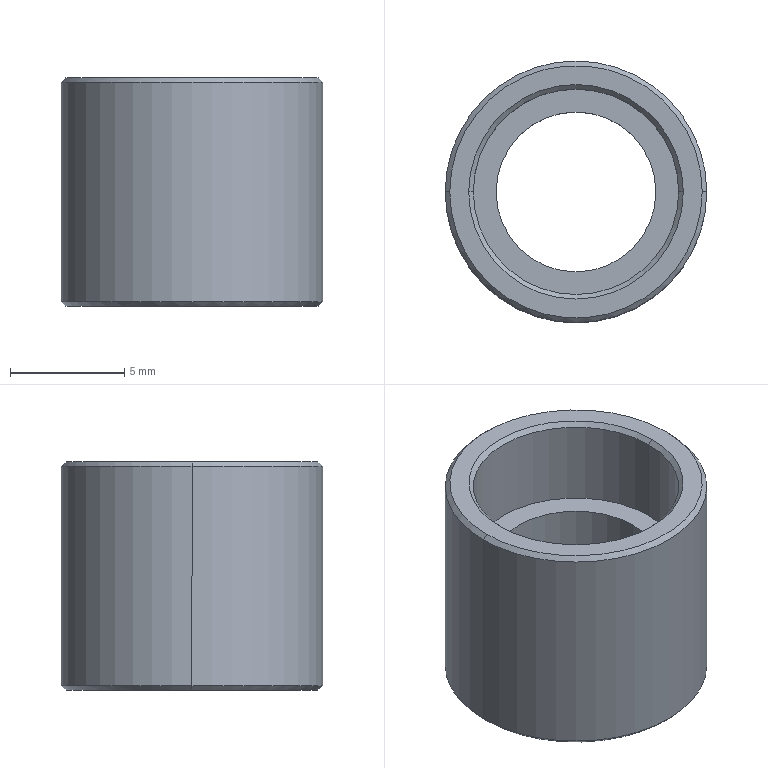Part | SolidWorks | features Revolution 1 | 1 solid | 20 faces | box 11.46 x 11.46 x 10 mm | volume 442.998 mm3 | cylinder 8 | cone 8 | plane 4 | commonest cylinder face diameters 9 x4 7 x2 11.46 x2
STEP:
#1=CARTESIAN_POINT('',(-4.5,0.,-9.8));
#2=VERTEX_POINT('',#1);
#3=CARTESIAN_POINT('',(4.5,0.,-9.8));
#4=VERTEX_POINT('',#3);
#5=CARTESIAN_POINT('',(0.,0.,-9.8));
#6=DIRECTION('',(0.,0.,1.));
#7=DIRECTION('',(1.,0.,0.));
#8=AXIS2_PLACEMENT_3D('',#5,#6,#7);
#9=CIRCLE('',#8,4.5);
#10=EDGE_CURVE('',#2,#4,#9,.T.);
#11=ORIENTED_EDGE('',*,*,#10,.F.);
#12=CARTESIAN_POINT('',(-4.5,0.,-6.));
#13=VERTEX_POINT('',#12);
#14=CARTESIAN_POINT('',(-4.5,0.,0.));
#15=DIRECTION('',(0.,0.,1.));
#16=VECTOR('',#15,1000.);
#17=LINE('',#14,#16);
#18=EDGE_CURVE('',#2,#13,#17,.T.);
#19=ORIENTED_EDGE('',*,*,#18,.T.);
#20=CARTESIAN_POINT('',(4.5,0.,-6.));
#21=VERTEX_POINT('',#20);
#22=CARTESIAN_POINT('',(0.,0.,-6.));
#23=DIRECTION('',(0.,0.,1.));
#24=DIRECTION('',(1.,0.,0.));
#25=AXIS2_PLACEMENT_3D('',#22,#23,#24);
#26=CIRCLE('',#25,4.5);
#27=EDGE_CURVE('',#13,#21,#26,.T.);
#28=ORIENTED_EDGE('',*,*,#27,.T.);
#29=CARTESIAN_POINT('',(4.5,0.,0.));
#30=DIRECTION('',(0.,0.,1.));
#31=VECTOR('',#30,1000.);
#32=LINE('',#29,#31);
#33=EDGE_CURVE('',#4,#21,#32,.T.);
#34=ORIENTED_EDGE('',*,*,#33,.F.);
#35=EDGE_LOOP('',(#11,#19,#28,#34));
#36=FACE_OUTER_BOUND('',#35,.T.);
#37=CARTESIAN_POINT('',(0.,0.,0.));
#38=DIRECTION('',(0.,0.,1.));
#39=DIRECTION('',(1.,0.,0.));
#40=AXIS2_PLACEMENT_3D('',#37,#38,#39);
#41=CYLINDRICAL_SURFACE('',#40,4.5);
#42=ADVANCED_FACE('',(#36),#41,.F.);
#43=ORIENTED_EDGE('',*,*,#10,.T.);
#44=CARTESIAN_POINT('',(4.7,0.,-10.));
#45=VERTEX_POINT('',#44);
#46=CARTESIAN_POINT('',(4.7,0.,-10.));
#47=DIRECTION('',(0.7071,0.,-0.7071));
#48=VECTOR('',#47,1000.);
#49=LINE('',#46,#48);
#50=EDGE_CURVE('',#4,#45,#49,.T.);
#51=ORIENTED_EDGE('',*,*,#50,.T.);
#52=CARTESIAN_POINT('',(-4.7,0.,-10.));
#53=VERTEX_POINT('',#52);
#54=CARTESIAN_POINT('',(0.,0.,-10.));
#55=DIRECTION('',(0.,0.,1.));
#56=DIRECTION('',(1.,0.,0.));
#57=AXIS2_PLACEMENT_3D('',#54,#55,#56);
#58=CIRCLE('',#57,4.7);
#59=EDGE_CURVE('',#53,#45,#58,.T.);
#60=ORIENTED_EDGE('',*,*,#59,.F.);
#61=CARTESIAN_POINT('',(-4.7,0.,-10.));
#62=DIRECTION('',(-0.7071,0.,-0.7071));
#63=VECTOR('',#62,1000.);
#64=LINE('',#61,#63);
#65=EDGE_CURVE('',#2,#53,#64,.T.);
#66=ORIENTED_EDGE('',*,*,#65,.F.);
#67=EDGE_LOOP('',(#43,#51,#60,#66));
#68=FACE_OUTER_BOUND('',#67,.T.);
#69=CARTESIAN_POINT('',(0.,0.,-10.));
#70=DIRECTION('',(0.,0.,-1.));
#71=DIRECTION('',(-1.,0.,0.));
#72=AXIS2_PLACEMENT_3D('',#69,#70,#71);
#73=CONICAL_SURFACE('',#72,4.7,0.7854);
#74=ADVANCED_FACE('',(#68),#73,.F.);
#75=CARTESIAN_POINT('',(5.53,0.,-10.));
#76=VERTEX_POINT('',#75);
#77=CARTESIAN_POINT('',(-5.53,0.,-10.));
#78=VERTEX_POINT('',#77);
#79=CARTESIAN_POINT('',(0.,0.,-10.));
#80=DIRECTION('',(0.,0.,1.));
#81=DIRECTION('',(1.,0.,0.));
#82=AXIS2_PLACEMENT_3D('',#79,#80,#81);
#83=CIRCLE('',#82,5.53);
#84=EDGE_CURVE('',#76,#78,#83,.T.);
#85=ORIENTED_EDGE('',*,*,#84,.T.);
#86=CARTESIAN_POINT('',(-5.73,0.,-9.8));
#87=VERTEX_POINT('',#86);
#88=CARTESIAN_POINT('',(-5.73,0.,-9.8));
#89=DIRECTION('',(-0.7071,0.,0.7071));
#90=VECTOR('',#89,1000.);
#91=LINE('',#88,#90);
#92=EDGE_CURVE('',#78,#87,#91,.T.);
#93=ORIENTED_EDGE('',*,*,#92,.T.);
#94=CARTESIAN_POINT('',(5.73,0.,-9.8));
#95=VERTEX_POINT('',#94);
#96=CARTESIAN_POINT('',(0.,0.,-9.8));
#97=DIRECTION('',(0.,0.,1.));
#98=DIRECTION('',(1.,0.,0.));
#99=AXIS2_PLACEMENT_3D('',#96,#97,#98);
#100=CIRCLE('',#99,5.73);
#101=EDGE_CURVE('',#95,#87,#100,.T.);
#102=ORIENTED_EDGE('',*,*,#101,.F.);
#103=CARTESIAN_POINT('',(5.73,0.,-9.8));
#104=DIRECTION('',(0.7071,0.,0.7071));
#105=VECTOR('',#104,1000.);
#106=LINE('',#103,#105);
#107=EDGE_CURVE('',#76,#95,#106,.T.);
#108=ORIENTED_EDGE('',*,*,#107,.F.);
#109=EDGE_LOOP('',(#85,#93,#102,#108));
#110=FACE_OUTER_BOUND('',#109,.T.);
#111=CARTESIAN_POINT('',(0.,0.,-9.8));
#112=DIRECTION('',(0.,0.,1.));
#113=DIRECTION('',(1.,0.,0.));
#114=AXIS2_PLACEMENT_3D('',#111,#112,#113);
#115=CONICAL_SURFACE('',#114,5.73,0.7854);
#116=ADVANCED_FACE('',(#110),#115,.T.);
#117=ORIENTED_EDGE('',*,*,#101,.T.);
#118=CARTESIAN_POINT('',(-5.73,0.,-0.2));
#119=VERTEX_POINT('',#118);
#120=CARTESIAN_POINT('',(-5.73,0.,0.));
#121=DIRECTION('',(0.,0.,1.));
#122=VECTOR('',#121,1000.);
#123=LINE('',#120,#122);
#124=EDGE_CURVE('',#87,#119,#123,.T.);
#125=ORIENTED_EDGE('',*,*,#124,.T.);
#126=CARTESIAN_POINT('',(5.73,0.,-0.2));
#127=VERTEX_POINT('',#126);
#128=CARTESIAN_POINT('',(0.,0.,-0.2));
#129=DIRECTION('',(0.,0.,1.));
#130=DIRECTION('',(1.,0.,0.));
#131=AXIS2_PLACEMENT_3D('',#128,#129,#130);
#132=CIRCLE('',#131,5.73);
#133=EDGE_CURVE('',#127,#119,#132,.T.);
#134=ORIENTED_EDGE('',*,*,#133,.F.);
#135=CARTESIAN_POINT('',(5.73,0.,0.));
#136=DIRECTION('',(0.,0.,1.));
#137=VECTOR('',#136,1000.);
#138=LINE('',#135,#137);
#139=EDGE_CURVE('',#95,#127,#138,.T.);
#140=ORIENTED_EDGE('',*,*,#139,.F.);
#141=EDGE_LOOP('',(#117,#125,#134,#140));
#142=FACE_OUTER_BOUND('',#141,.T.);
#143=CARTESIAN_POINT('',(0.,0.,0.));
#144=DIRECTION('',(0.,0.,1.));
#145=DIRECTION('',(1.,0.,0.));
#146=AXIS2_PLACEMENT_3D('',#143,#144,#145);
#147=CYLINDRICAL_SURFACE('',#146,5.73);
#148=ADVANCED_FACE('',(#142),#147,.T.);
#149=CARTESIAN_POINT('',(5.53,0.,0.));
#150=VERTEX_POINT('',#149);
#151=CARTESIAN_POINT('',(-5.53,0.,0.));
#152=VERTEX_POINT('',#151);
#153=CARTESIAN_POINT('',(0.,0.,0.));
#154=DIRECTION('',(0.,0.,1.));
#155=DIRECTION('',(1.,0.,0.));
#156=AXIS2_PLACEMENT_3D('',#153,#154,#155);
#157=CIRCLE('',#156,5.53);
#158=EDGE_CURVE('',#150,#152,#157,.T.);
#159=ORIENTED_EDGE('',*,*,#158,.F.);
#160=CARTESIAN_POINT('',(5.53,0.,0.));
#161=DIRECTION('',(0.7071,0.,-0.7071));
#162=VECTOR('',#161,1000.);
#163=LINE('',#160,#162);
#164=EDGE_CURVE('',#150,#127,#163,.T.);
#165=ORIENTED_EDGE('',*,*,#164,.T.);
#166=ORIENTED_EDGE('',*,*,#133,.T.);
#167=CARTESIAN_POINT('',(-5.53,0.,0.));
#168=DIRECTION('',(-0.7071,0.,-0.7071));
#169=VECTOR('',#168,1000.);
#170=LINE('',#167,#169);
#171=EDGE_CURVE('',#152,#119,#170,.T.);
#172=ORIENTED_EDGE('',*,*,#171,.F.);
#173=EDGE_LOOP('',(#159,#165,#166,#172));
#174=FACE_OUTER_BOUND('',#173,.T.);
#175=CARTESIAN_POINT('',(0.,0.,0.));
#176=DIRECTION('',(0.,0.,-1.));
#177=DIRECTION('',(-1.,0.,0.));
#178=AXIS2_PLACEMENT_3D('',#175,#176,#177);
#179=CONICAL_SURFACE('',#178,5.53,0.7854);
#180=ADVANCED_FACE('',(#174),#179,.T.);
#181=CARTESIAN_POINT('',(-4.5,0.,-0.2));
#182=VERTEX_POINT('',#181);
#183=CARTESIAN_POINT('',(4.5,0.,-0.2));
#184=VERTEX_POINT('',#183);
#185=CARTESIAN_POINT('',(0.,0.,-0.2));
#186=DIRECTION('',(0.,0.,1.));
#187=DIRECTION('',(1.,0.,0.));
#188=AXIS2_PLACEMENT_3D('',#185,#186,#187);
#189=CIRCLE('',#188,4.5);
#190=EDGE_CURVE('',#182,#184,#189,.T.);
#191=ORIENTED_EDGE('',*,*,#190,.F.);
#192=CARTESIAN_POINT('',(-4.7,0.,0.));
#193=VERTEX_POINT('',#192);
#194=CARTESIAN_POINT('',(-4.5,0.,-0.2));
#195=DIRECTION('',(-0.7071,0.,0.7071));
#196=VECTOR('',#195,1000.);
#197=LINE('',#194,#196);
#198=EDGE_CURVE('',#182,#193,#197,.T.);
#199=ORIENTED_EDGE('',*,*,#198,.T.);
#200=CARTESIAN_POINT('',(4.7,0.,0.));
#201=VERTEX_POINT('',#200);
#202=CARTESIAN_POINT('',(0.,0.,0.));
#203=DIRECTION('',(0.,0.,1.));
#204=DIRECTION('',(1.,0.,0.));
#205=AXIS2_PLACEMENT_3D('',#202,#203,#204);
#206=CIRCLE('',#205,4.7);
#207=EDGE_CURVE('',#193,#201,#206,.T.);
#208=ORIENTED_EDGE('',*,*,#207,.T.);
#209=CARTESIAN_POINT('',(4.5,0.,-0.2));
#210=DIRECTION('',(0.7071,0.,0.7071));
#211=VECTOR('',#210,1000.);
#212=LINE('',#209,#211);
#213=EDGE_CURVE('',#184,#201,#212,.T.);
#214=ORIENTED_EDGE('',*,*,#213,.F.);
#215=EDGE_LOOP('',(#191,#199,#208,#214));
#216=FACE_OUTER_BOUND('',#215,.T.);
#217=CARTESIAN_POINT('',(0.,0.,-0.2));
#218=DIRECTION('',(0.,0.,1.));
#219=DIRECTION('',(1.,0.,0.));
#220=AXIS2_PLACEMENT_3D('',#217,#218,#219);
#221=CONICAL_SURFACE('',#220,4.5,0.7854);
#222=ADVANCED_FACE('',(#216),#221,.F.);
#223=CARTESIAN_POINT('',(-4.5,0.,-4.));
#224=VERTEX_POINT('',#223);
#225=CARTESIAN_POINT('',(4.5,0.,-4.));
#226=VERTEX_POINT('',#225);
#227=CARTESIAN_POINT('',(0.,0.,-4.));
#228=DIRECTION('',(0.,0.,1.));
#229=DIRECTION('',(1.,0.,0.));
#230=AXIS2_PLACEMENT_3D('',#227,#228,#229);
#231=CIRCLE('',#230,4.5);
#232=EDGE_CURVE('',#224,#226,#231,.T.);
#233=ORIENTED_EDGE('',*,*,#232,.F.);
#234=CARTESIAN_POINT('',(-4.5,0.,0.));
#235=DIRECTION('',(0.,0.,1.));
#236=VECTOR('',#235,1000.);
#237=LINE('',#234,#236);
#238=EDGE_CURVE('',#224,#182,#237,.T.);
#239=ORIENTED_EDGE('',*,*,#238,.T.);
#240=ORIENTED_EDGE('',*,*,#190,.T.);
#241=CARTESIAN_POINT('',(4.5,0.,0.));
#242=DIRECTION('',(0.,0.,1.));
#243=VECTOR('',#242,1000.);
#244=LINE('',#241,#243);
#245=EDGE_CURVE('',#226,#184,#244,.T.);
#246=ORIENTED_EDGE('',*,*,#245,.F.);
#247=EDGE_LOOP('',(#233,#239,#240,#246));
#248=FACE_OUTER_BOUND('',#247,.T.);
#249=CARTESIAN_POINT('',(0.,0.,0.));
#250=DIRECTION('',(0.,0.,1.));
#251=DIRECTION('',(1.,0.,0.));
#252=AXIS2_PLACEMENT_3D('',#249,#250,#251);
#253=CYLINDRICAL_SURFACE('',#252,4.5);
#254=ADVANCED_FACE('',(#248),#253,.F.);
#255=CARTESIAN_POINT('',(-3.5,0.,-6.));
#256=VERTEX_POINT('',#255);
#257=CARTESIAN_POINT('',(3.5,0.,-6.));
#258=VERTEX_POINT('',#257);
#259=CARTESIAN_POINT('',(0.,0.,-6.));
#260=DIRECTION('',(0.,0.,1.));
#261=DIRECTION('',(1.,0.,0.));
#262=AXIS2_PLACEMENT_3D('',#259,#260,#261);
#263=CIRCLE('',#262,3.5);
#264=EDGE_CURVE('',#256,#258,#263,.T.);
#265=ORIENTED_EDGE('',*,*,#264,.F.);
#266=CARTESIAN_POINT('',(-3.5,0.,-4.));
#267=VERTEX_POINT('',#266);
#268=CARTESIAN_POINT('',(-3.5,0.,0.));
#269=DIRECTION('',(0.,0.,1.));
#270=VECTOR('',#269,1000.);
#271=LINE('',#268,#270);
#272=EDGE_CURVE('',#256,#267,#271,.T.);
#273=ORIENTED_EDGE('',*,*,#272,.T.);
#274=CARTESIAN_POINT('',(3.5,0.,-4.));
#275=VERTEX_POINT('',#274);
#276=CARTESIAN_POINT('',(0.,0.,-4.));
#277=DIRECTION('',(0.,0.,1.));
#278=DIRECTION('',(1.,0.,0.));
#279=AXIS2_PLACEMENT_3D('',#276,#277,#278);
#280=CIRCLE('',#279,3.5);
#281=EDGE_CURVE('',#267,#275,#280,.T.);
#282=ORIENTED_EDGE('',*,*,#281,.T.);
#283=CARTESIAN_POINT('',(3.5,0.,0.));
#284=DIRECTION('',(0.,0.,1.));
#285=VECTOR('',#284,1000.);
#286=LINE('',#283,#285);
#287=EDGE_CURVE('',#258,#275,#286,.T.);
#288=ORIENTED_EDGE('',*,*,#287,.F.);
#289=EDGE_LOOP('',(#265,#273,#282,#288));
#290=FACE_OUTER_BOUND('',#289,.T.);
#291=CARTESIAN_POINT('',(0.,0.,0.));
#292=DIRECTION('',(0.,0.,1.));
#293=DIRECTION('',(1.,0.,0.));
#294=AXIS2_PLACEMENT_3D('',#291,#292,#293);
#295=CYLINDRICAL_SURFACE('',#294,3.5);
#296=ADVANCED_FACE('',(#290),#295,.F.);
#297=CARTESIAN_POINT('',(0.,0.,-6.));
#298=DIRECTION('',(0.,0.,1.));
#299=DIRECTION('',(1.,0.,0.));
#300=AXIS2_PLACEMENT_3D('',#297,#298,#299);
#301=CIRCLE('',#300,3.5);
#302=EDGE_CURVE('',#258,#256,#301,.T.);
#303=ORIENTED_EDGE('',*,*,#302,.T.);
#304=ORIENTED_EDGE('',*,*,#264,.T.);
#305=EDGE_LOOP('',(#303,#304));
#306=FACE_BOUND('',#305,.T.);
#307=CARTESIAN_POINT('',(0.,0.,-6.));
#308=DIRECTION('',(0.,0.,1.));
#309=DIRECTION('',(1.,0.,0.));
#310=AXIS2_PLACEMENT_3D('',#307,#308,#309);
#311=CIRCLE('',#310,4.5);
#312=EDGE_CURVE('',#21,#13,#311,.T.);
#313=ORIENTED_EDGE('',*,*,#312,.F.);
#314=ORIENTED_EDGE('',*,*,#27,.F.);
#315=EDGE_LOOP('',(#313,#314));
#316=FACE_OUTER_BOUND('',#315,.T.);
#317=CARTESIAN_POINT('',(4.5,0.,-6.));
#318=DIRECTION('',(0.,0.,-1.));
#319=DIRECTION('',(-1.,0.,0.));
#320=AXIS2_PLACEMENT_3D('',#317,#318,#319);
#321=PLANE('',#320);
#322=ADVANCED_FACE('',(#306,#316),#321,.T.);
#323=ORIENTED_EDGE('',*,*,#272,.F.);
#324=ORIENTED_EDGE('',*,*,#302,.F.);
#325=ORIENTED_EDGE('',*,*,#287,.T.);
#326=CARTESIAN_POINT('',(0.,0.,-4.));
#327=DIRECTION('',(0.,0.,1.));
#328=DIRECTION('',(1.,0.,0.));
#329=AXIS2_PLACEMENT_3D('',#326,#327,#328);
#330=CIRCLE('',#329,3.5);
#331=EDGE_CURVE('',#275,#267,#330,.T.);
#332=ORIENTED_EDGE('',*,*,#331,.T.);
#333=EDGE_LOOP('',(#323,#324,#325,#332));
#334=FACE_OUTER_BOUND('',#333,.T.);
#335=CARTESIAN_POINT('',(0.,0.,0.));
#336=DIRECTION('',(0.,0.,1.));
#337=DIRECTION('',(1.,0.,0.));
#338=AXIS2_PLACEMENT_3D('',#335,#336,#337);
#339=CYLINDRICAL_SURFACE('',#338,3.5);
#340=ADVANCED_FACE('',(#334),#339,.F.);
#341=CARTESIAN_POINT('',(0.,0.,-4.));
#342=DIRECTION('',(0.,0.,1.));
#343=DIRECTION('',(1.,0.,0.));
#344=AXIS2_PLACEMENT_3D('',#341,#342,#343);
#345=CIRCLE('',#344,4.5);
#346=EDGE_CURVE('',#226,#224,#345,.T.);
#347=ORIENTED_EDGE('',*,*,#346,.T.);
#348=ORIENTED_EDGE('',*,*,#232,.T.);
#349=EDGE_LOOP('',(#347,#348));
#350=FACE_OUTER_BOUND('',#349,.T.);
#351=ORIENTED_EDGE('',*,*,#331,.F.);
#352=ORIENTED_EDGE('',*,*,#281,.F.);
#353=EDGE_LOOP('',(#351,#352));
#354=FACE_BOUND('',#353,.T.);
#355=CARTESIAN_POINT('',(3.5,0.,-4.));
#356=DIRECTION('',(0.,0.,1.));
#357=DIRECTION('',(1.,0.,0.));
#358=AXIS2_PLACEMENT_3D('',#355,#356,#357);
#359=PLANE('',#358);
#360=ADVANCED_FACE('',(#350,#354),#359,.T.);
#361=ORIENTED_EDGE('',*,*,#238,.F.);
#362=ORIENTED_EDGE('',*,*,#346,.F.);
#363=ORIENTED_EDGE('',*,*,#245,.T.);
#364=CARTESIAN_POINT('',(0.,0.,-0.2));
#365=DIRECTION('',(0.,0.,1.));
#366=DIRECTION('',(1.,0.,0.));
#367=AXIS2_PLACEMENT_3D('',#364,#365,#366);
#368=CIRCLE('',#367,4.5);
#369=EDGE_CURVE('',#184,#182,#368,.T.);
#370=ORIENTED_EDGE('',*,*,#369,.T.);
#371=EDGE_LOOP('',(#361,#362,#363,#370));
#372=FACE_OUTER_BOUND('',#371,.T.);
#373=CARTESIAN_POINT('',(0.,0.,0.));
#374=DIRECTION('',(0.,0.,1.));
#375=DIRECTION('',(1.,0.,0.));
#376=AXIS2_PLACEMENT_3D('',#373,#374,#375);
#377=CYLINDRICAL_SURFACE('',#376,4.5);
#378=ADVANCED_FACE('',(#372),#377,.F.);
#379=ORIENTED_EDGE('',*,*,#198,.F.);
#380=ORIENTED_EDGE('',*,*,#369,.F.);
#381=ORIENTED_EDGE('',*,*,#213,.T.);
#382=CARTESIAN_POINT('',(0.,0.,0.));
#383=DIRECTION('',(0.,0.,1.));
#384=DIRECTION('',(1.,0.,0.));
#385=AXIS2_PLACEMENT_3D('',#382,#383,#384);
#386=CIRCLE('',#385,4.7);
#387=EDGE_CURVE('',#201,#193,#386,.T.);
#388=ORIENTED_EDGE('',*,*,#387,.T.);
#389=EDGE_LOOP('',(#379,#380,#381,#388));
#390=FACE_OUTER_BOUND('',#389,.T.);
#391=CARTESIAN_POINT('',(0.,0.,-0.2));
#392=DIRECTION('',(0.,0.,1.));
#393=DIRECTION('',(1.,0.,0.));
#394=AXIS2_PLACEMENT_3D('',#391,#392,#393);
#395=CONICAL_SURFACE('',#394,4.5,0.7854);
#396=ADVANCED_FACE('',(#390),#395,.F.);
#397=CARTESIAN_POINT('',(0.,0.,0.));
#398=DIRECTION('',(0.,0.,1.));
#399=DIRECTION('',(1.,0.,0.));
#400=AXIS2_PLACEMENT_3D('',#397,#398,#399);
#401=CIRCLE('',#400,5.53);
#402=EDGE_CURVE('',#152,#150,#401,.T.);
#403=ORIENTED_EDGE('',*,*,#402,.T.);
#404=ORIENTED_EDGE('',*,*,#158,.T.);
#405=EDGE_LOOP('',(#403,#404));
#406=FACE_OUTER_BOUND('',#405,.T.);
#407=ORIENTED_EDGE('',*,*,#387,.F.);
#408=ORIENTED_EDGE('',*,*,#207,.F.);
#409=EDGE_LOOP('',(#407,#408));
#410=FACE_BOUND('',#409,.T.);
#411=CARTESIAN_POINT('',(4.7,0.,0.));
#412=DIRECTION('',(0.,0.,1.));
#413=DIRECTION('',(1.,0.,0.));
#414=AXIS2_PLACEMENT_3D('',#411,#412,#413);
#415=PLANE('',#414);
#416=ADVANCED_FACE('',(#406,#410),#415,.T.);
#417=ORIENTED_EDGE('',*,*,#164,.F.);
#418=ORIENTED_EDGE('',*,*,#402,.F.);
#419=ORIENTED_EDGE('',*,*,#171,.T.);
#420=CARTESIAN_POINT('',(0.,0.,-0.2));
#421=DIRECTION('',(0.,0.,1.));
#422=DIRECTION('',(1.,0.,0.));
#423=AXIS2_PLACEMENT_3D('',#420,#421,#422);
#424=CIRCLE('',#423,5.73);
#425=EDGE_CURVE('',#119,#127,#424,.T.);
#426=ORIENTED_EDGE('',*,*,#425,.T.);
#427=EDGE_LOOP('',(#417,#418,#419,#426));
#428=FACE_OUTER_BOUND('',#427,.T.);
#429=CARTESIAN_POINT('',(0.,0.,0.));
#430=DIRECTION('',(0.,0.,-1.));
#431=DIRECTION('',(-1.,0.,0.));
#432=AXIS2_PLACEMENT_3D('',#429,#430,#431);
#433=CONICAL_SURFACE('',#432,5.53,0.7854);
#434=ADVANCED_FACE('',(#428),#433,.T.);
#435=ORIENTED_EDGE('',*,*,#124,.F.);
#436=CARTESIAN_POINT('',(0.,0.,-9.8));
#437=DIRECTION('',(0.,0.,1.));
#438=DIRECTION('',(1.,0.,0.));
#439=AXIS2_PLACEMENT_3D('',#436,#437,#438);
#440=CIRCLE('',#439,5.73);
#441=EDGE_CURVE('',#87,#95,#440,.T.);
#442=ORIENTED_EDGE('',*,*,#441,.T.);
#443=ORIENTED_EDGE('',*,*,#139,.T.);
#444=ORIENTED_EDGE('',*,*,#425,.F.);
#445=EDGE_LOOP('',(#435,#442,#443,#444));
#446=FACE_OUTER_BOUND('',#445,.T.);
#447=CARTESIAN_POINT('',(0.,0.,0.));
#448=DIRECTION('',(0.,0.,1.));
#449=DIRECTION('',(1.,0.,0.));
#450=AXIS2_PLACEMENT_3D('',#447,#448,#449);
#451=CYLINDRICAL_SURFACE('',#450,5.73);
#452=ADVANCED_FACE('',(#446),#451,.T.);
#453=ORIENTED_EDGE('',*,*,#92,.F.);
#454=CARTESIAN_POINT('',(0.,0.,-10.));
#455=DIRECTION('',(0.,0.,1.));
#456=DIRECTION('',(1.,0.,0.));
#457=AXIS2_PLACEMENT_3D('',#454,#455,#456);
#458=CIRCLE('',#457,5.53);
#459=EDGE_CURVE('',#78,#76,#458,.T.);
#460=ORIENTED_EDGE('',*,*,#459,.T.);
#461=ORIENTED_EDGE('',*,*,#107,.T.);
#462=ORIENTED_EDGE('',*,*,#441,.F.);
#463=EDGE_LOOP('',(#453,#460,#461,#462));
#464=FACE_OUTER_BOUND('',#463,.T.);
#465=CARTESIAN_POINT('',(0.,0.,-9.8));
#466=DIRECTION('',(0.,0.,1.));
#467=DIRECTION('',(1.,0.,0.));
#468=AXIS2_PLACEMENT_3D('',#465,#466,#467);
#469=CONICAL_SURFACE('',#468,5.73,0.7854);
#470=ADVANCED_FACE('',(#464),#469,.T.);
#471=ORIENTED_EDGE('',*,*,#59,.T.);
#472=CARTESIAN_POINT('',(0.,0.,-10.));
#473=DIRECTION('',(0.,0.,1.));
#474=DIRECTION('',(1.,0.,0.));
#475=AXIS2_PLACEMENT_3D('',#472,#473,#474);
#476=CIRCLE('',#475,4.7);
#477=EDGE_CURVE('',#45,#53,#476,.T.);
#478=ORIENTED_EDGE('',*,*,#477,.T.);
#479=EDGE_LOOP('',(#471,#478));
#480=FACE_BOUND('',#479,.T.);
#481=ORIENTED_EDGE('',*,*,#84,.F.);
#482=ORIENTED_EDGE('',*,*,#459,.F.);
#483=EDGE_LOOP('',(#481,#482));
#484=FACE_OUTER_BOUND('',#483,.T.);
#485=CARTESIAN_POINT('',(5.53,0.,-10.));
#486=DIRECTION('',(0.,0.,-1.));
#487=DIRECTION('',(-1.,0.,0.));
#488=AXIS2_PLACEMENT_3D('',#485,#486,#487);
#489=PLANE('',#488);
#490=ADVANCED_FACE('',(#480,#484),#489,.T.);
#491=ORIENTED_EDGE('',*,*,#50,.F.);
#492=CARTESIAN_POINT('',(0.,0.,-9.8));
#493=DIRECTION('',(0.,0.,1.));
#494=DIRECTION('',(1.,0.,0.));
#495=AXIS2_PLACEMENT_3D('',#492,#493,#494);
#496=CIRCLE('',#495,4.5);
#497=EDGE_CURVE('',#4,#2,#496,.T.);
#498=ORIENTED_EDGE('',*,*,#497,.T.);
#499=ORIENTED_EDGE('',*,*,#65,.T.);
#500=ORIENTED_EDGE('',*,*,#477,.F.);
#501=EDGE_LOOP('',(#491,#498,#499,#500));
#502=FACE_OUTER_BOUND('',#501,.T.);
#503=CARTESIAN_POINT('',(0.,0.,-10.));
#504=DIRECTION('',(0.,0.,-1.));
#505=DIRECTION('',(-1.,0.,0.));
#506=AXIS2_PLACEMENT_3D('',#503,#504,#505);
#507=CONICAL_SURFACE('',#506,4.7,0.7854);
#508=ADVANCED_FACE('',(#502),#507,.F.);
#509=ORIENTED_EDGE('',*,*,#18,.F.);
#510=ORIENTED_EDGE('',*,*,#497,.F.);
#511=ORIENTED_EDGE('',*,*,#33,.T.);
#512=ORIENTED_EDGE('',*,*,#312,.T.);
#513=EDGE_LOOP('',(#509,#510,#511,#512));
#514=FACE_OUTER_BOUND('',#513,.T.);
#515=CARTESIAN_POINT('',(0.,0.,0.));
#516=DIRECTION('',(0.,0.,1.));
#517=DIRECTION('',(1.,0.,0.));
#518=AXIS2_PLACEMENT_3D('',#515,#516,#517);
#519=CYLINDRICAL_SURFACE('',#518,4.5);
#520=ADVANCED_FACE('',(#514),#519,.F.);
#521=CLOSED_SHELL('',(#42,#74,#116,#148,#180,#222,#254,#296,#322,#340,#360,#378,#396,#416,#434,#452,#470,#490,#508,#520));
#522=MANIFOLD_SOLID_BREP('',#521);
#523=CARTESIAN_POINT('',(0.,0.,0.));
#524=DIRECTION('',(0.,0.,1.));
#525=DIRECTION('',(1.,0.,0.));
#526=AXIS2_PLACEMENT_3D('',#523,#524,#525);
#527=(LENGTH_UNIT()NAMED_UNIT(*)SI_UNIT(.MILLI.,.METRE.));
#528=UNCERTAINTY_MEASURE_WITH_UNIT(LENGTH_MEASURE(0.00001),#527,'','');
#529=(NAMED_UNIT(*)PLANE_ANGLE_UNIT()SI_UNIT($,.RADIAN.));
#530=(NAMED_UNIT(*)SI_UNIT($,.STERADIAN.)SOLID_ANGLE_UNIT());
#531=(GEOMETRIC_REPRESENTATION_CONTEXT(3)GLOBAL_UNCERTAINTY_ASSIGNED_CONTEXT((#528))GLOBAL_UNIT_ASSIGNED_CONTEXT((#527,#529,#530))REPRESENTATION_CONTEXT('',''));
#532=ADVANCED_BREP_SHAPE_REPRESENTATION('',(#522,#526),#531);